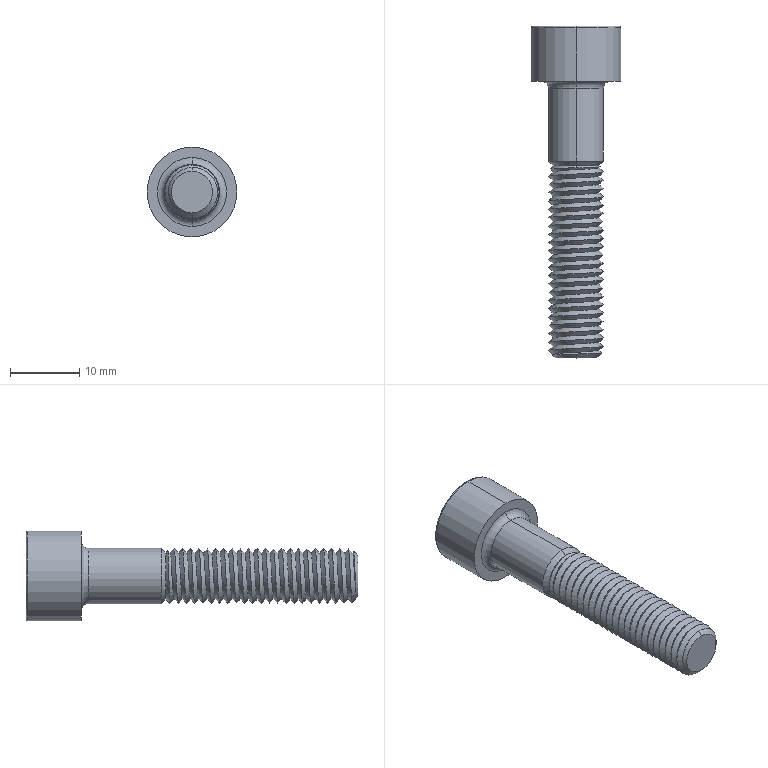Part | STEP file | Parafuso M8 - 40mm | 1 solid | 36 faces | box 13 x 48 x 13 mm | volume 2619 mm3 | plane 16 | cone 8 | torus 6 | cylinder 4 | spline 2 | commonest cylinder face diameters 8 x2 13 x2